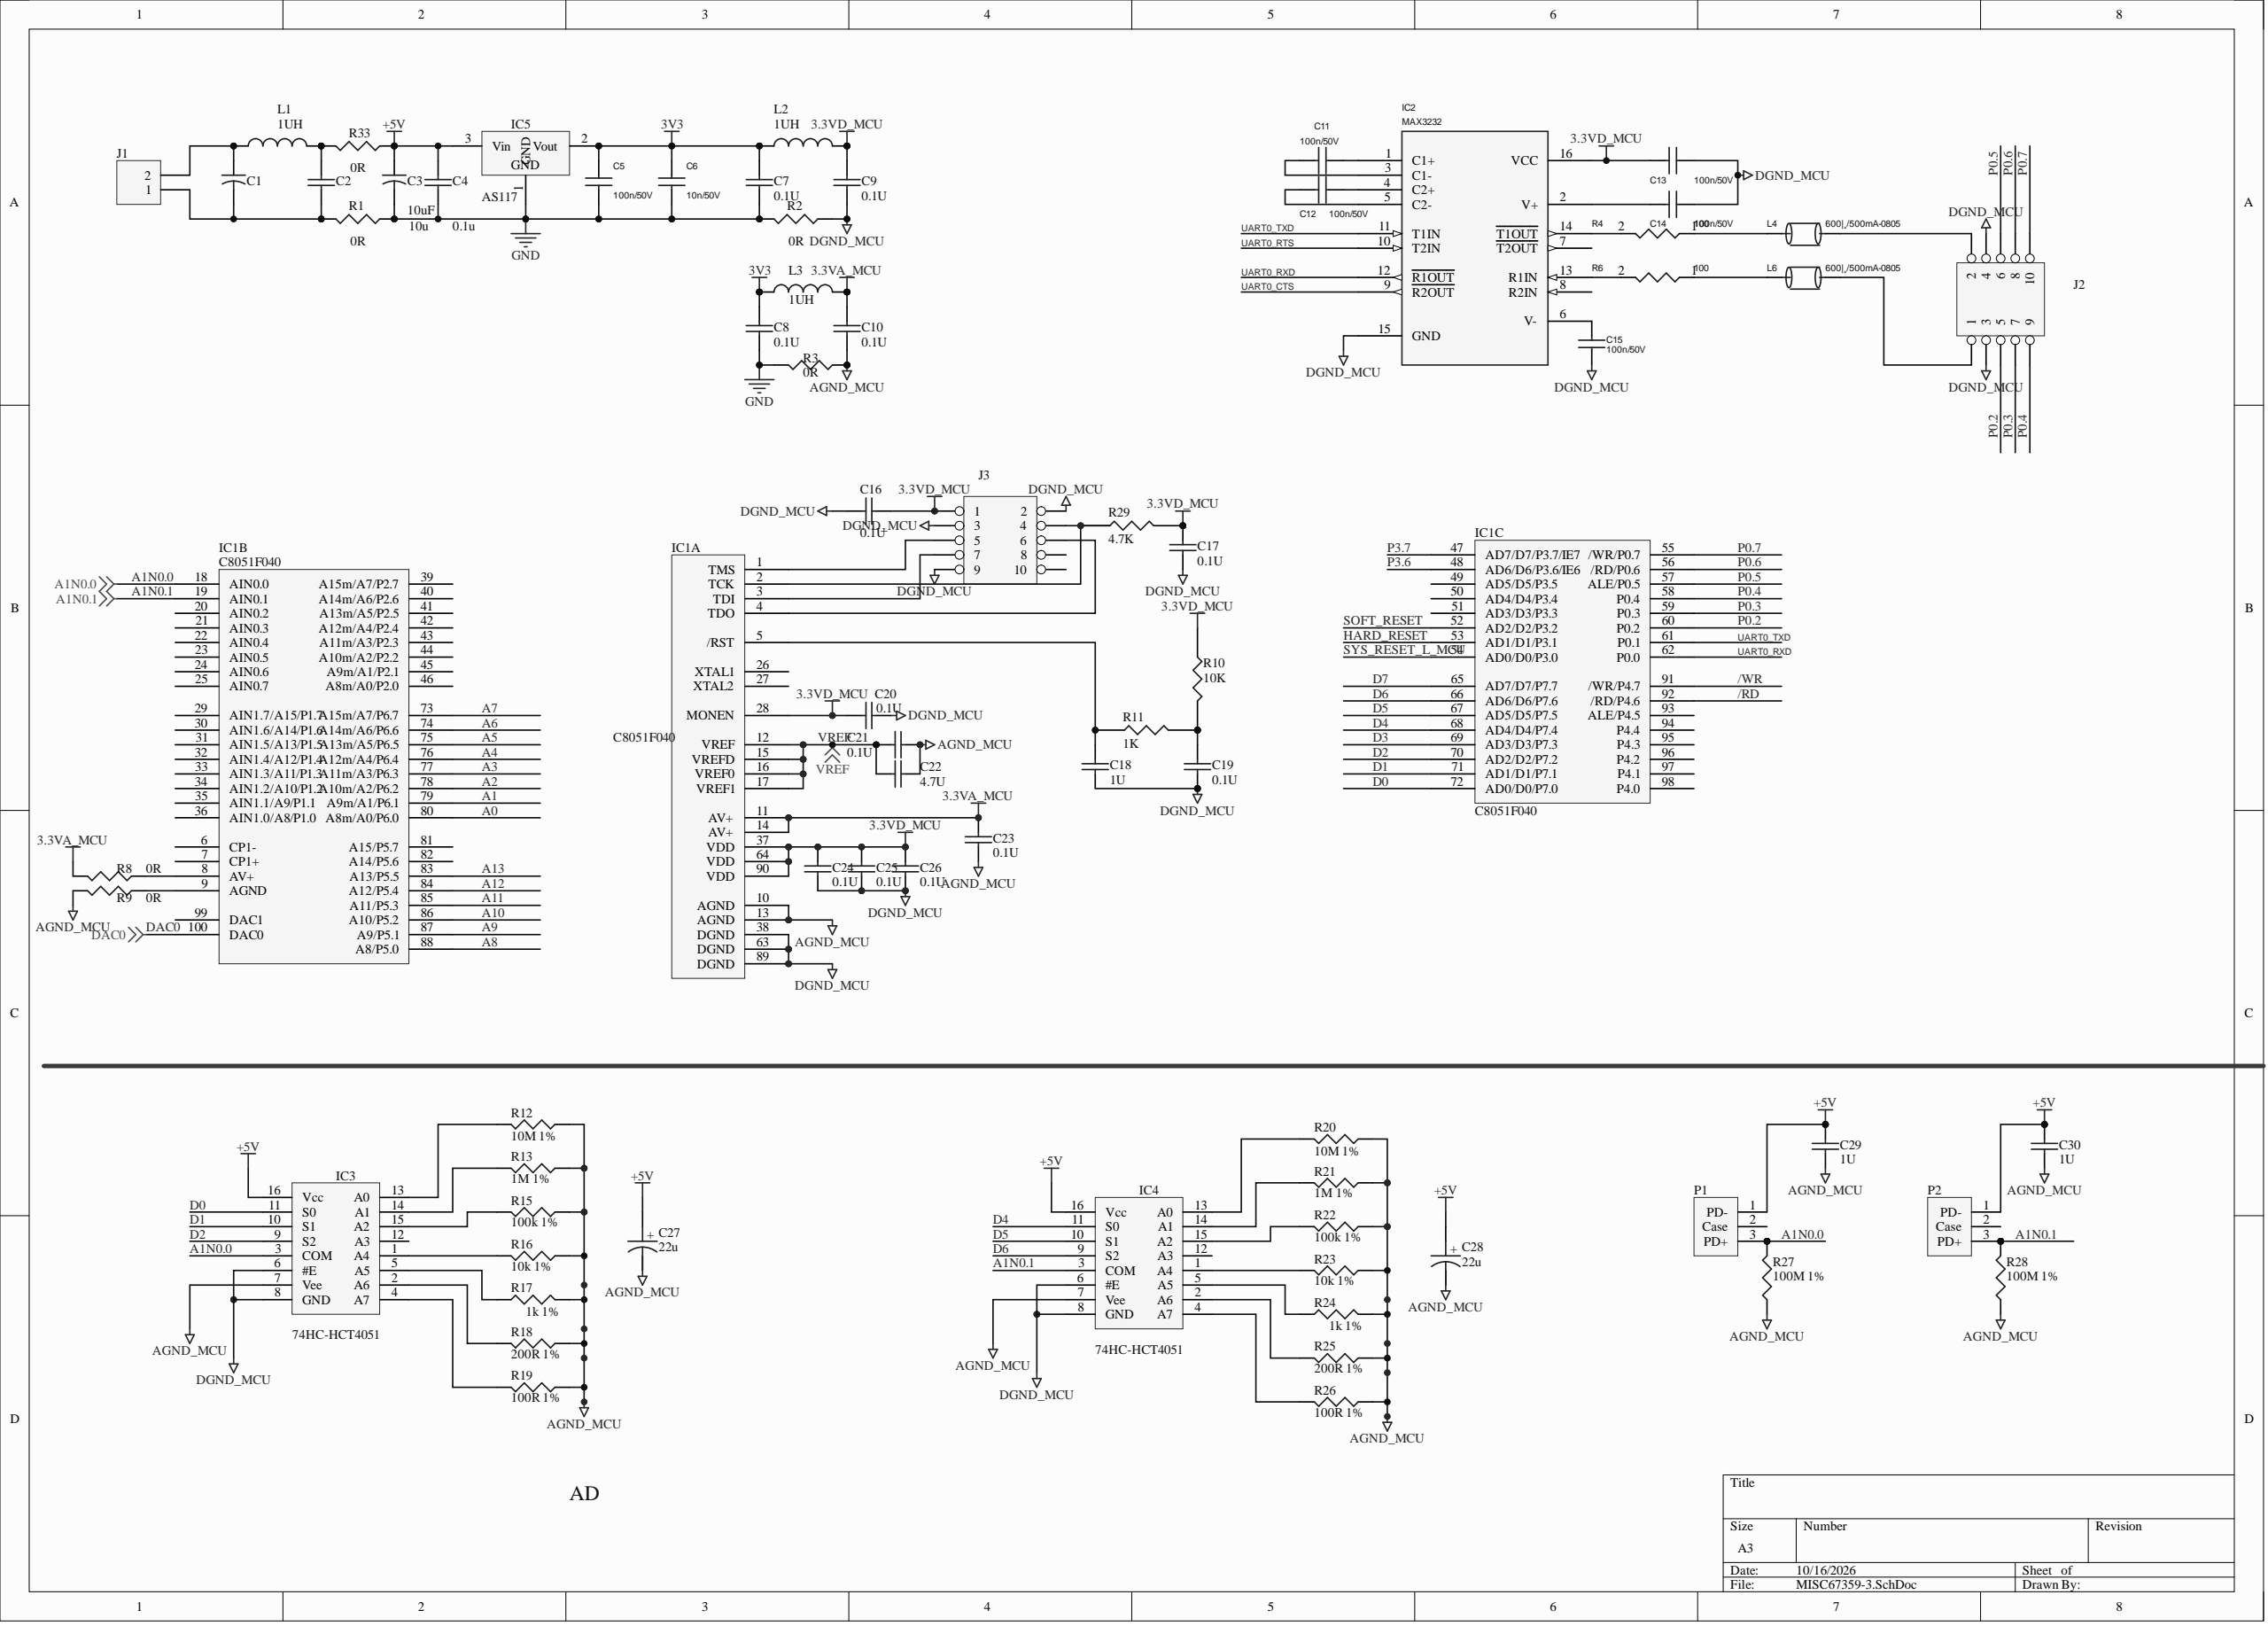Circuit board | Altium Designer | 72 parts | 61 nets
Bill of materials:
Comment,Description,Designator,Footprint,LibRef,Quantity
"","Capacitor","C1, C2","CAPC3216N","Cap2, CAP","2"
"10u","Capacitor","C3","CAPC2012N","Cap2","1"
"0.1u","Capacitor","C4, C7, C8, C9, C10, C16, C17, C19, C20, C21, C23, C24, C25, C26","0603","CAP","14"
"100n/50V","","C5, C11, C12, C13, C14, C15","0603","CAPACITOR NON-POL","6"
"10n/50V","","C6","0603","CAPACITOR NON-POL","1"
"1U","Capacitor","C18, C29, C30","0603","CAP","3"
"4.7U","Capacitor","C22","0603","CAP","1"
"22u","","C27, C28","3528","CAPACITOR POL","2"
"C8051F040","","IC1","TQFP100","C8051F020","1"
"MAX3232","","IC2","SOIC127P600-16N","MAX3232","1"
"74HC-HCT4051","","IC3, IC4","SOIC16","CD54HC4051","2"
"AS117","Voltage Regulator","IC5","SOT89L","Volt Reg","1"
"","Header, 2-Pin","J1","MKDS3_2RMI","Header 2","1"
"","","J2, J3","FKV10SN","HEADER 5X2","2"
"1UH","","L1, L2, L3","0805","INDUCTOR","3"
"600|¸/500mA-0805","","L4, L6","0805","BEAD","2"
"","","P1, P2","E3","MHDR1X3","2"
"0R","Resistor","R1, R2, R3, R33","6-0805_N","RES","4"
"100","","R4, R6","0603","SMDRXX_2","2"
"0R","Resistor","R8, R9","0603","RES","2"
"10K","","R10","0603","RES1","1"
"1K","","R11","0603","RES1","1"
"10M 1%","","R12, R20","0603","RES1","2"
"1M 1%","","R13, R21","0603","RES1","2"
"100k 1%","","R15, R22","0603","RES1","2"
"10k 1%","","R16, R23","0603","RES1","2"
"1k 1%","","R17, R24","0603","RES1","2"
"200R 1%","","R18, R25","0603","RES1","2"
"100R 1%","","R19, R26","0603","RES1","2"
"100M 1%","","R27, R28","0603","RES1","2"
"4.7K","","R29","0603","RES1","1"
Netlist (Protel format):
[
C1
CAPC3216N




]
[
C2
CAPC3216N




]
[
C3
CAPC2012N
10u



]
[
C4
0603
0.1u



]
[
C5
0603
100n/50V



]
[
C6
0603
10n/50V



]
[
C7
0603
0.1U



]
[
C8
0603
0.1U



]
[
C9
0603
0.1U



]
[
C10
0603
0.1U



]
[
C11
0603
100n/50V



]
[
C12
0603
100n/50V



]
[
C13
0603
100n/50V



]
[
C14
0603
100n/50V



]
[
C15
0603
100n/50V



]
[
C16
0603
0.1U



]
[
C17
0603
0.1U



]
[
C18
0603
1U



]
[
C19
0603
0.1U



]
[
C20
0603
0.1U



]
[
C21
0603
0.1U



]
[
C22
0603
4.7U



]
[
C23
0603
0.1U



]
[
C24
0603
0.1U



]
[
C25
0603
0.1U



]
[
C26
0603
0.1U



]
[
C27
3528
22u



]
[
C28
3528
22u



]
[
C29
0603
1U



]
[
C30
0603
1U



]
[
IC1
TQFP100
C8051F040



]
[
IC2
SOIC127P600-16N
MAX3232



]
[
IC3
SOIC16
74HC-HCT4051



]
[
IC4
SOIC16
74HC-HCT4051



]
[
IC5
SOT89L
AS117



]
[
J1
MKDS3_2RMI




]
[
J2
FKV10SN




]
[
J3
FKV10SN




]
[
L1
0805
1UH



]
[
L2
0805
1UH



]
[
L3
0805
1UH



]
[
L4
0805
600|¸/500mA-0805



]
[
L6
0805
600|¸/500mA-0805



]
[
P1
E3




]
[
P2
E3




]
[
R1
6-0805_N
0R



]
[
R2
6-0805_N
0R



]
[
R3
6-0805_N
0R



]
[
R4
0603
100



]
[
R6
0603
100



]
[
R8
0603
0R



]
[
R9
0603
0R



]
[
R10
0603
10K



]
[
R11
0603
1K



]
[
R12
0603
10M 1%



]
[
R13
0603
1M 1%



]
[
R15
0603
100k 1%



]
[
R16
0603
10k 1%



]
[
R17
0603
1k 1%



]
[
R18
0603
200R 1%



]
[
R19
0603
100R 1%



]
[
R20
0603
10M 1%



]
[
R21
0603
1M 1%



]
[
R22
0603
100k 1%



]
[
R23
0603
10k 1%



]
[
R24
0603
1k 1%



]
[
R25
0603
200R 1%



]
[
R26
0603
100R 1%



]
[
R27
0603
100M 1%



]
[
R28
0603
100M 1%



]
[
R29
0603
4.7K



]
[
R33
6-0805_N
0R



]
(
VREF
C21-2
C22-2
IC1-12
IC1-15
IC1-16
IC1-17
)
(
UART0_TXD
IC1-61
IC2-11
)
(
UART0_RXD
IC1-62
IC2-12
)
(
P0.7
IC1-55
J2-10
)
(
P0.6
IC1-56
J2-8
)
(
P0.5
IC1-57
J2-6
)
(
P0.4
IC1-58
J2-9
)
(
P0.3
IC1-59
J2-7
)
(
P0.2
IC1-60
J2-5
)
(
NetL6_1
L6-1
R6-1
)
(
NetL4_1
L4-1
R4-1
)
(
NetJ2_2
J2-2
L4-2
)
(
NetJ2_1
J2-1
L6-2
)
(
NetIC4_15
IC4-15
R22-2
)
(
NetIC4_14
IC4-14
R21-2
)
(
NetIC4_13
IC4-13
R20-2
)
(
NetIC4_5
IC4-5
R24-1
)
(
NetIC4_4
IC4-4
R26-2
)
(
NetIC4_2
IC4-2
R25-2
)
(
NetIC4_1
IC4-1
R23-2
)
(
NetIC3_15
IC3-15
R15-2
)
(
NetIC3_14
IC3-14
R13-2
)
(
NetIC3_13
IC3-13
R12-2
)
(
NetIC3_5
IC3-5
R17-1
)
(
NetIC3_4
IC3-4
R19-2
)
(
NetIC3_2
IC3-2
R18-2
)
(
NetIC3_1
IC3-1
R16-2
)
(
NetIC2_14
IC2-14
R4-2
)
(
NetIC2_13
IC2-13
R6-2
)
(
NetIC1_9
IC1-9
R9-2
)
(
NetIC1_8
IC1-8
R8-2
)
(
NetIC1_4
IC1-4
J3-6
)
(
NetIC1_3
IC1-3
J3-7
)
(
NetIC1_2
IC1-2
J3-4
R29-2
)
(
NetIC1_1
IC1-1
J3-5
)
(
NetC19_2
C19-2
R10-1
R11-1
)
(
NetC18_2
C18-2
IC1-5
R11-2
)
(
NetC15_2
C15-2
IC2-6
)
(
NetC14_2
C14-2
IC2-2
)
(
NetC12_2
C12-2
IC2-5
)
(
NetC12_1
C12-1
IC2-4
)
(
NetC11_2
C11-2
IC2-3
)
(
NetC11_1
C11-1
IC2-1
)
(
NetC2_1
C2-1
L1-2
R33-1
)
(
NetC1_2
C1-2
C2-2
J1-1
R1-1
)
(
NetC1_1
C1-1
J1-2
L1-1
)
(
GND
C3-2
C4-2
C5-2
C6-2
C7-1
C8-1
IC5-1
R1-2
R2-1
R3-1
)
(
DGND_MCU
C9-2
C13-1
C14-1
C15-1
C16-1
C17-2
C18-1
C19-1
C20-1
C24-1
C25-1
C26-1
IC1-38
IC1-63
IC1-89
IC2-15
IC3-6
IC3-8
IC4-6
IC4-8
J2-3
J2-4
J3-2
J3-3
J3-9
R2-2
)
(
D6
IC1-66
IC4-9
)
(
D5
IC1-67
IC4-10
)
(
D4
IC1-68
IC4-11
)
(
D2
IC1-70
IC3-9
)
(
D1
IC1-71
IC3-10
)
(
D0
IC1-72
IC3-11
)
(
AGND_MCU
C10-2
C21-1
C22-1
C23-1
C27-2
C28-2
C29-1
C30-1
IC1-10
IC1-13
IC3-7
IC4-7
R3-2
R9-1
R12-1
R13-1
R15-1
R16-1
R17-2
R18-1
R19-1
R20-1
R21-1
R22-1
R23-1
R24-2
R25-1
R26-1
R27-1
R28-1
)
(
A1N0.1
IC1-19
IC4-3
P2-3
R28-2
)
(
A1N0.0
IC1-18
IC3-3
P1-3
R27-2
)
(
+5V
C3-1
C4-1
C27-1
C28-1
C29-2
C30-2
IC3-16
IC4-16
IC5-3
P1-1
P2-1
R33-2
)
(
3V3
C5-1
C6-1
C7-2
C8-2
IC5-2
L2-1
L3-2
)
(
3.3VD_MCU
C9-1
C13-2
C16-2
C17-1
C20-2
C24-2
C25-2
C26-2
IC1-28
IC1-37
IC1-64
IC1-90
IC2-16
J3-1
L2-2
R10-2
R29-1
)
(
3.3VA_MCU
C10-1
C23-2
IC1-11
IC1-14
L3-1
R8-1
)